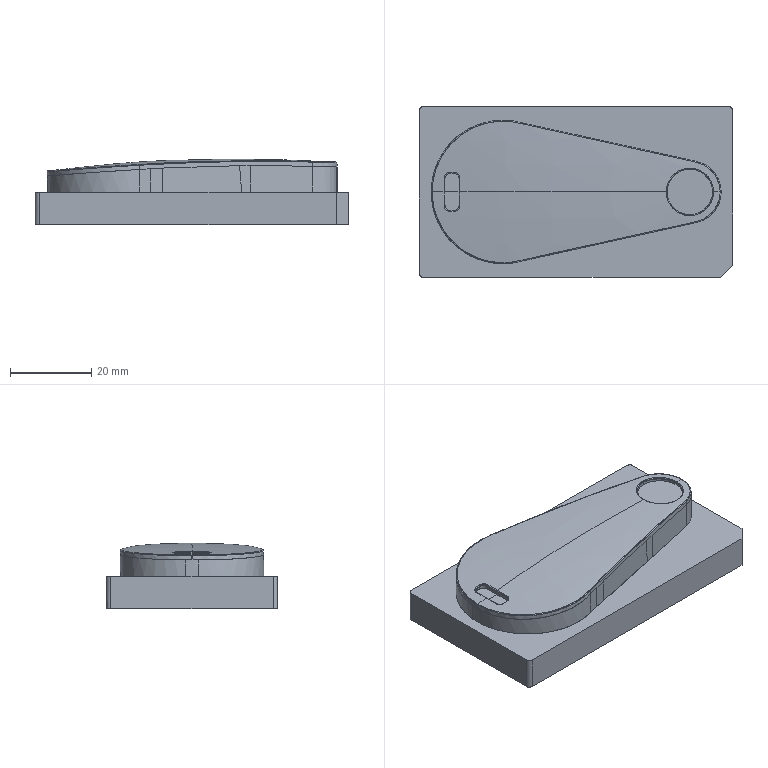NC program | PowerMill | posted with a generic post | part box 77 x 42 x 16.114 mm
Lines 17525 to 19132 of 230441, first 1450 of 1608 lines:
N17622 M6
N17623 S18000 M03
N17624 G00 G90 X0.0 Y0.0
N17625 G43 Z9.8037 H28
N17626
N17627 G05 P10000 R4
N17628 X-29.8878 Y2.5312
N17629 Z-1.421
N17630 G01 Z-2.621 F2400.0
N17631 X-29.8713 Y2.5316 F4000.0
N17632 G03 X-29.726 Y2.6832 I-0.0032 J0.1484
N17633 G01 X-29.7401 Y3.336
N17634 X-29.7435 Y3.3599
N17635 X-29.7525 Y3.3822
N17636 X-29.8269 Y3.5167
N17637 X-29.8421 Y3.5374
N17638 X-29.8621 Y3.5535
N17639 X-29.9916 Y3.633
N17640 X-30.0319 Y3.647
N17641 X-30.5975 Y3.7149
N17642 X-29.8892 Y2.3639 Z-2.7177
N17643 X-29.8727
N17644 G03 X-29.7242 Y2.5124 I0.0 J0.1485
N17645 G01 Y2.5785
N17646 X-29.7405 Y3.335
N17647 X-29.7439 Y3.359
N17648 X-29.753 Y3.3814
N17649 X-29.8258 Y3.5126
N17650 X-29.8424 Y3.5347
N17651 X-29.8644 Y3.5514
N17652 X-29.9942 Y3.6241
N17653 X-30.0167 Y3.6334
N17654 X-30.0408 Y3.6369
N17655 X-30.827 Y3.6548
N17656 G00 Z1.579
N17657 G01 X-30.7616 Y-3.5711 F10000.0
N17658 G00 Z-1.421
N17659 G01 Z-2.621 F2400.0
N17660 X-30.7596 Y-3.5875 F4000.0
N17661 G03 X-30.5941 Y-3.7167 I0.1474 J0.0182
N17662 G01 X-30.0322 Y-3.6476
N17663 X-29.9918 Y-3.6335
N17664 X-29.8615 Y-3.553
N17665 X-29.8417 Y-3.5368
N17666 X-29.8266 Y-3.5162
N17667 X-29.7519 Y-3.3811
N17668 X-29.7431 Y-3.3596
N17669 X-29.7263 Y-3.0196
N17670 X-29.7252 Y-2.6792
N17671 X-30.9888 Y-3.4914 Z-2.7177
N17672 X-30.9886 Y-3.5079
N17673 G03 X-30.8387 Y-3.655 I0.1485 J0.0014
N17674 G01 X-30.0951 Y-3.6479
N17675 X-29.9745 Y-3.6175
N17676 X-29.9604 Y-3.6128
N17677 X-29.9472 Y-3.606
N17678 X-29.9065 Y-3.5808
N17679 X-29.8454 Y-3.5337
N17680 X-29.831 Y-3.5201
N17681 X-29.8196 Y-3.5038
N17682 X-29.7549 Y-3.3866
N17683 X-29.7484 Y-3.3722
N17684 X-29.7444 Y-3.3569
N17685 X-29.7248 Y-2.9283
N17686 X-29.7249 Y-2.4993
N17687 X-31.2076 Y-2.5192 Z-2.6145
N17688 X-31.2074 Y-3.3335 Z-2.6287 F2400.0
N17689 X-31.1952 Y-3.373 Z-2.6294
N17690 X-31.097 Y-3.5168 Z-2.6325
N17691 X-31.0697 Y-3.5403 Z-2.6331
N17692 X-30.9489 Y-3.599 Z-2.6354
N17693 X-30.9192 Y-3.606 Z-2.636
N17694 X-30.0987 Y-3.6169 Z-2.6503
N17695 X-29.9719 Y-3.5858 Z-2.6526
N17696 X-29.9713 Y-3.5856
N17697 X-29.924 Y-3.5564 Z-2.6535
N17698 X-29.8574 Y-3.5051 Z-2.655
N17699 X-29.8521 Y-3.5006 Z-2.6551
N17700 X-29.7781 Y-3.3667 Z-2.6578
N17701 X-29.7752 Y-3.3606 Z-2.6579
N17702 X-29.772 Y-3.3426 Z-2.6582
N17703 X-29.7555 Y-2.9522 Z-2.6651
N17704 X-29.7549 Y-2.4993 Z-2.673
N17705 X-29.7542 Y-2.0587 Z-2.6806
N17706 Y-0.6131 Z-2.7059
N17707 X-29.9539 Z-2.7094
N17708 X-30.3986 Y-0.7228 Z-2.7174
N17709 X-30.8042 Y-0.9356 Z-2.7253
N17710 X-31.147 Y-1.2394 Z-2.7333
N17711 X-31.2079 Y-1.3275 Z-2.7352
N17712 X-31.2074 Y-3.3335 Z-2.7702
N17713 X-31.1952 Y-3.373 Z-2.7709
N17714 X-31.097 Y-3.5168 Z-2.774
N17715 X-31.0697 Y-3.5403 Z-2.7746
N17716 X-30.9489 Y-3.599 Z-2.7769
N17717 X-30.9192 Y-3.606 Z-2.7775
N17718 X-30.0987 Y-3.6169 Z-2.7918
N17719 X-29.9719 Y-3.5858 Z-2.7941
N17720 X-29.9713 Y-3.5856
N17721 X-29.924 Y-3.5564 Z-2.7951
N17722 X-29.8574 Y-3.5051 Z-2.7965
N17723 X-29.8521 Y-3.5006 Z-2.7966
N17724 X-29.7781 Y-3.3667 Z-2.7993
N17725 X-29.7752 Y-3.3606 Z-2.7994
N17726 X-29.772 Y-3.3426 Z-2.7998
N17727 X-29.7555 Y-2.9522 Z-2.8066
N17728 X-29.7549 Y-2.4993 Z-2.8145
N17729 X-29.7249
N17730 X-29.7242 Y-2.0587 F4000.0
N17731 Y2.5785
N17732 X-29.7243 Y2.5825
N17733 X-29.7398 Y3.3077
N17734 X-29.7659 Y3.4048
N17735 X-29.8139 Y3.4913
N17736 X-29.8799 Y3.5601
N17737 X-29.9667 Y3.6088
N17738 X-30.0627 Y3.6374
N17739 X-30.3495 Y3.644
N17740 X-30.919 Y3.6369
N17741 X-30.9413 Y3.6341
N17742 X-30.9624 Y3.6264
N17743 X-31.0855 Y3.5651
N17744 X-31.1064 Y3.5511
N17745 X-31.1232 Y3.5324
N17746 X-31.2212 Y3.3903
N17747 X-31.2344 Y3.3632
N17748 X-31.2389 Y3.3335
N17749 X-31.2374 Y-3.3335
N17750 X-31.2329 Y-3.363
N17751 X-31.22 Y-3.3899
N17752 X-31.1218 Y-3.5337
N17753 X-31.1045 Y-3.5531
N17754 X-31.0828 Y-3.5673
N17755 X-30.9619 Y-3.626
N17756 X-30.9413 Y-3.6333
N17757 X-30.9197 Y-3.636
N17758 X-30.0953 Y-3.647
N17759 X-29.9648 Y-3.6149
N17760 X-29.9619 Y-3.6142
N17761 X-29.959 Y-3.6133
N17762 X-29.907 Y-3.5811
N17763 X-29.8391 Y-3.5289
N17764 X-29.8334 Y-3.5242
N17765 X-29.8281 Y-3.519
N17766 X-29.8272 Y-3.5177
N17767 X-29.8265 Y-3.5163
N17768 X-29.7519 Y-3.3812
N17769 X-29.7493 Y-3.3762
N17770 X-29.747 Y-3.3711
N17771 X-29.7436 Y-3.3577
N17772 X-29.742 Y-3.3438
N17773 X-29.7255 Y-2.9528
N17774 X-29.7249 Y-2.4993
N17775 X-31.1785 Y-2.4363 Z-2.7112
N17776 X-31.1788 Y-3.2629 Z-2.7257 F2400.0
N17777 X-31.1515 Y-3.3898 Z-2.7279
N17778 X-31.1378 Y-3.4188 Z-2.7285
N17779 X-31.0478 Y-3.5314 Z-2.731
N17780 X-30.9867 Y-3.5716 Z-2.7323
N17781 X-30.956 Y-3.5828 Z-2.7329
N17782 X-30.7255 Y-3.6086 Z-2.7369
N17783 X-30.0989 Y-3.617 Z-2.7478
N17784 X-29.9719 Y-3.5858 Z-2.7501
N17785 X-29.9711 Y-3.5856
N17786 X-29.9245 Y-3.5568 Z-2.7511
N17787 X-29.8574 Y-3.5051 Z-2.7526
N17788 X-29.852 Y-3.5005 Z-2.7527
N17789 X-29.7781 Y-3.3667 Z-2.7554
N17790 X-29.7753 Y-3.3611 Z-2.7555
N17791 X-29.772 Y-3.3426 Z-2.7558
N17792 X-29.7555 Y-2.9507 Z-2.7626
N17793 X-29.7548 Y-2.4993 Z-2.7705
N17794 X-29.7542 Y-2.1026 Z-2.7774
N17795 Y-0.6131 Z-2.8034
N17796 X-29.9538 Z-2.8069
N17797 X-30.3986 Y-0.7228 Z-2.8149
N17798 X-30.8041 Y-0.9356 Z-2.8229
N17799 X-31.147 Y-1.2394 Z-2.8309
N17800 X-31.1782 Y-1.2845 Z-2.8319
N17801 X-31.1788 Y-3.2629 Z-2.8664
N17802 X-31.1515 Y-3.3898 Z-2.8687
N17803 X-31.1378 Y-3.4188 Z-2.8692
N17804 X-31.0478 Y-3.5314 Z-2.8717
N17805 X-30.9867 Y-3.5716 Z-2.873
N17806 X-30.956 Y-3.5828 Z-2.8736
N17807 X-30.7255 Y-3.6086 Z-2.8776
N17808 X-30.0989 Y-3.617 Z-2.8886
N17809 X-29.9719 Y-3.5858 Z-2.8908
N17810 X-29.9711 Y-3.5856 Z-2.8909
N17811 X-29.9245 Y-3.5568 Z-2.8918
N17812 X-29.8574 Y-3.5051 Z-2.8933
N17813 X-29.852 Y-3.5005 Z-2.8934
N17814 X-29.7781 Y-3.3667 Z-2.8961
N17815 X-29.7753 Y-3.3611 Z-2.8962
N17816 X-29.772 Y-3.3426 Z-2.8965
N17817 X-29.7555 Y-2.9507 Z-2.9034
N17818 X-29.7548 Y-2.4993 Z-2.9112
N17819 X-29.7248
N17820 X-29.7242 Y-2.1027 F4000.0
N17821 X-29.7243 Y2.5785
N17822 X-29.7399 Y3.3081
N17823 X-29.7658 Y3.4044
N17824 X-29.8141 Y3.4916
N17825 X-29.8794 Y3.5597
N17826 X-29.9684 Y3.6093
N17827 X-30.0617 Y3.6372
N17828 X-30.103 Y3.6384
N17829 X-30.3495 Y3.644
N17830 X-30.7191 Y3.6394
N17831 X-30.9522 Y3.6133
N17832 X-30.9811 Y3.6056
N17833 X-31.0065 Y3.5896
N17834 X-31.1417 Y3.4724
N17835 X-31.185 Y3.3872
N17836 X-31.193 Y3.3655
N17837 X-31.1959 Y3.3427
N17838 X-31.2071 Y1.8909
N17839 X-31.2088 Y-3.2661
N17840 X-31.1809 Y-3.3961
N17841 X-31.1734 Y-3.418
N17842 X-31.1612 Y-3.4376
N17843 X-31.0682 Y-3.5538
N17844 X-31.0032 Y-3.5967
N17845 X-30.9822 Y-3.6072
N17846 X-30.9593 Y-3.6126
N17847 X-30.7274 Y-3.6386
N17848 X-30.0973 Y-3.647
N17849 X-30.0952
N17850 X-29.9648 Y-3.6149
N17851 X-29.9618 Y-3.6141
N17852 X-29.9588 Y-3.6133
N17853 X-29.9074 Y-3.5815
N17854 X-29.8391 Y-3.5289
N17855 X-29.8333 Y-3.5241
N17856 X-29.8279 Y-3.5189
N17857 X-29.8272 Y-3.5176
N17858 X-29.8264 Y-3.5163
N17859 X-29.7518 Y-3.3812
N17860 X-29.7494 Y-3.3765
N17861 X-29.7472 Y-3.3718
N17862 X-29.7436 Y-3.358
N17863 X-29.742 Y-3.3438
N17864 X-29.7255 Y-2.9513
N17865 X-29.7248 Y-2.4993
N17866 X-31.1716 Y-2.4142 Z-2.808
N17867 Y-2.5782 Z-2.8109 F2400.0
N17868 X-31.1549 Y-3.359 Z-2.8245
N17869 X-31.1199 Y-3.4375 Z-2.826
N17870 X-31.1026 Y-3.4612 Z-2.8265
N17871 X-30.985 Y-3.5663 Z-2.8292
N17872 X-30.9462 Y-3.5836 Z-2.83
N17873 X-30.7242 Y-3.6087 Z-2.8339
N17874 X-30.0992 Y-3.617 Z-2.8448
N17875 X-30.0991
N17876 X-29.9719 Y-3.5858 Z-2.8471
N17877 X-29.9709 Y-3.5855
N17878 X-29.9249 Y-3.5571 Z-2.848
N17879 X-29.8574 Y-3.5051 Z-2.8495
N17880 X-29.8519 Y-3.5004 Z-2.8497
N17881 X-29.778 Y-3.3667 Z-2.8523
N17882 X-29.7755 Y-3.3616 Z-2.8524
N17883 X-29.772 Y-3.3426 Z-2.8528
N17884 X-29.7554 Y-2.9492 Z-2.8596
N17885 X-29.7548 Y-2.4993 Z-2.8675
N17886 X-29.7543 Y-2.1452 Z-2.8737
N17887 Y-0.6131 Z-2.9004
N17888 X-29.9538 Z-2.9039
N17889 X-30.3985 Y-0.7228 Z-2.9119
N17890 X-30.8041 Y-0.9356 Z-2.9199
N17891 X-31.1469 Y-1.2394 Z-2.9279
N17892 X-31.1712 Y-1.2746 Z-2.9286
N17893 X-31.1716 Y-2.5782 Z-2.9514
N17894 X-31.1549 Y-3.359 Z-2.965
N17895 X-31.1199 Y-3.4375 Z-2.9665
N17896 X-31.1026 Y-3.4612 Z-2.967
N17897 X-30.985 Y-3.5663 Z-2.9698
N17898 X-30.9462 Y-3.5836 Z-2.9705
N17899 X-30.7242 Y-3.6087 Z-2.9744
N17900 X-30.0992 Y-3.617 Z-2.9853
N17901 X-30.0991
N17902 X-29.9719 Y-3.5858 Z-2.9876
N17903 X-29.9709 Y-3.5855
N17904 X-29.9249 Y-3.5571 Z-2.9886
N17905 X-29.8574 Y-3.5051 Z-2.99
N17906 X-29.8519 Y-3.5004 Z-2.9902
N17907 X-29.778 Y-3.3667 Z-2.9928
N17908 X-29.7755 Y-3.3616 Z-2.9929
N17909 X-29.772 Y-3.3426 Z-2.9933
N17910 X-29.7554 Y-2.9492 Z-3.0001
N17911 X-29.7548 Y-2.4993 Z-3.008
N17912 X-29.7248
N17913 X-29.7243 Y-2.1453 F4000.0
N17914 Y2.5785
N17915 X-29.7399 Y3.3083
N17916 X-29.7657 Y3.4042
N17917 X-29.8142 Y3.4918
N17918 X-29.8793 Y3.5596
N17919 X-29.9686 Y3.6095
N17920 X-30.0616 Y3.6372
N17921 X-30.1102 Y3.6386
N17922 X-30.3495 Y3.6441
N17923 X-30.7179 Y3.6395
N17924 X-30.9496 Y3.6135
N17925 X-30.9793 Y3.6054
N17926 X-31.0051 Y3.5886
N17927 X-31.1177 Y3.4878
N17928 X-31.1354 Y3.467
N17929 X-31.1468 Y3.4422
N17930 X-31.1964 Y3.2778
N17931 X-31.2001 Y2.8058
N17932 X-31.2016 Y-2.5785
N17933 X-31.1847 Y-3.3656
N17934 X-31.1473 Y-3.4497
N17935 X-31.1367 Y-3.4679
N17936 X-31.1226 Y-3.4836
N17937 X-31.0049 Y-3.5887
N17938 X-30.9792 Y-3.6054
N17939 X-30.9495 Y-3.6135
N17940 X-30.726 Y-3.6387
N17941 X-30.0992 Y-3.647
N17942 X-30.0953
N17943 X-29.9648 Y-3.6149
N17944 X-29.9617 Y-3.6141
N17945 X-29.9586 Y-3.6132
N17946 X-29.9078 Y-3.5818
N17947 X-29.8391 Y-3.5289
N17948 X-29.8332 Y-3.524
N17949 X-29.8278 Y-3.5187
N17950 X-29.8271 Y-3.5175
N17951 X-29.8264 Y-3.5163
N17952 X-29.7518 Y-3.3812
N17953 X-29.7495 Y-3.3769
N17954 X-29.7475 Y-3.3724
N17955 X-29.7437 Y-3.3583
N17956 X-29.742 Y-3.3438
N17957 X-29.7254 Y-2.9498
N17958 X-29.7248 Y-2.4993
N17959 X-31.1714 Y-2.4074 Z-2.9047
N17960 Y-2.5784 Z-2.9077 F2400.0
N17961 X-31.1713 Y-2.5954 Z-2.908
N17962 X-31.1562 Y-3.2986 Z-2.9203
N17963 X-31.1168 Y-3.4349 Z-2.9228
N17964 X-31.1022 Y-3.4616 Z-2.9233
N17965 X-30.985 Y-3.5663 Z-2.9261
N17966 X-30.969 Y-3.5771 Z-2.9264
N17967 X-30.9463 Y-3.5836 Z-2.9268
N17968 X-30.7235 Y-3.6087 Z-2.9307
N17969 X-30.1012 Y-3.6171 Z-2.9416
N17970 X-30.0991 Y-3.617
N17971 X-29.9719 Y-3.5858 Z-2.9439
N17972 X-29.9708 Y-3.5855
N17973 X-29.9253 Y-3.5574 Z-2.9449
N17974 X-29.8574 Y-3.5051 Z-2.9464
N17975 X-29.8517 Y-3.5003 Z-2.9465
N17976 X-29.778 Y-3.3667 Z-2.9491
N17977 X-29.7756 Y-3.362 Z-2.9492
N17978 X-29.772 Y-3.3426 Z-2.9496
N17979 X-29.7554 Y-2.9476 Z-2.9565
N17980 X-29.7547 Y-2.4993 Z-2.9643
N17981 X-29.7543 Y-2.1892 Z-2.9697
N17982 Y-0.6131 Z-2.9972
N17983 X-29.9537 Z-3.0007
N17984 X-30.3985 Y-0.7228 Z-3.0087
N17985 X-30.804 Y-0.9356 Z-3.0167
N17986 X-31.1469 Y-1.2394 Z-3.0247
N17987 X-31.171 Y-1.2743 Z-3.0254
N17988 X-31.1714 Y-2.5784 Z-3.0482
N17989 X-31.1713 Y-2.5954 Z-3.0485
N17990 X-31.1562 Y-3.2986 Z-3.0608
N17991 X-31.1168 Y-3.4349 Z-3.0632
N17992 X-31.1022 Y-3.4616 Z-3.0638
N17993 X-30.985 Y-3.5663 Z-3.0665
N17994 X-30.969 Y-3.5771 Z-3.0668
N17995 X-30.9463 Y-3.5836 Z-3.0673
N17996 X-30.7235 Y-3.6087 Z-3.0712
N17997 X-30.1012 Y-3.6171 Z-3.082
N17998 X-30.0991 Y-3.617 Z-3.0821
N17999 X-29.9719 Y-3.5858 Z-3.0843
N18000 X-29.9708 Y-3.5855 Z-3.0844
N18001 X-29.9253 Y-3.5574 Z-3.0853
N18002 X-29.8574 Y-3.5051 Z-3.0868
N18003 X-29.8517 Y-3.5003 Z-3.0869
N18004 X-29.778 Y-3.3667 Z-3.0896
N18005 X-29.7756 Y-3.362 Z-3.0897
N18006 X-29.772 Y-3.3426 Z-3.09
N18007 X-29.7554 Y-2.9476 Z-3.0969
N18008 X-29.7547 Y-2.4993 Z-3.1047
N18009 X-29.7247
N18010 X-29.7243 Y-2.1892 F4000.0
N18011 Y2.5785
N18012 X-29.7399 Y3.3085
N18013 X-29.7656 Y3.404
N18014 X-29.8143 Y3.4919
N18015 X-29.8791 Y3.5595
N18016 X-29.9689 Y3.6096
N18017 X-30.0614 Y3.6372
N18018 X-30.1175 Y3.6388
N18019 X-30.3495 Y3.6441
N18020 X-30.7172 Y3.6396
N18021 X-30.9495 Y3.6135
N18022 X-30.9792 Y3.6054
N18023 X-31.0051 Y3.5886
N18024 X-31.1177 Y3.4878
N18025 X-31.1354 Y3.4669
N18026 X-31.1468 Y3.442
N18027 X-31.1965 Y3.2761
N18028 X-31.1996 Y2.8745
N18029 X-31.2014 Y-2.5785
N18030 X-31.2013 Y-2.5958
N18031 X-31.1861 Y-3.3032
N18032 X-31.1457 Y-3.4432
N18033 X-31.1369 Y-3.4643
N18034 X-31.1235 Y-3.4828
N18035 X-31.1231 Y-3.4832
N18036 X-31.1226 Y-3.4836
N18037 X-31.005 Y-3.5887
N18038 X-30.9941 Y-3.5972
N18039 X-30.9821 Y-3.604
N18040 X-30.9663 Y-3.6101
N18041 X-30.9497 Y-3.6134
N18042 X-30.7254 Y-3.6387
N18043 X-30.1012 Y-3.6471
N18044 X-30.0953 Y-3.647
N18045 X-29.9648 Y-3.6149
N18046 X-29.9616 Y-3.6141
N18047 X-29.9584 Y-3.6131
N18048 X-29.9083 Y-3.5821
N18049 X-29.8391 Y-3.5289
N18050 X-29.8332 Y-3.524
N18051 X-29.8276 Y-3.5186
N18052 X-29.8263 Y-3.5163
N18053 X-29.7517 Y-3.3812
N18054 X-29.7496 Y-3.3772
N18055 X-29.7477 Y-3.3731
N18056 X-29.7438 Y-3.3587
N18057 X-29.742 Y-3.3439
N18058 X-29.7254 Y-2.9483
N18059 X-29.7247 Y-2.4993
N18060 X-31.1713 Y-2.4064 Z-3.0015
N18061 X-31.1714 Y-2.5784 Z-3.0045 F2400.0
N18062 X-31.1712 Y-2.6002 Z-3.0049
N18063 X-31.1563 Y-3.2984 Z-3.0171
N18064 X-31.1168 Y-3.4349 Z-3.0195
N18065 X-31.102 Y-3.4618 Z-3.0201
N18066 X-30.9898 Y-3.5621 Z-3.0227
N18067 X-30.9849 Y-3.5664 Z-3.0228
N18068 X-30.9463 Y-3.5836 Z-3.0236
N18069 X-30.7229 Y-3.6088 Z-3.0275
N18070 X-30.1031 Y-3.6171 Z-3.0383
N18071 X-30.0991 Y-3.617 Z-3.0384
N18072 X-29.972 Y-3.5858 Z-3.0407
N18073 X-29.9706 Y-3.5854
N18074 X-29.9258 Y-3.5577 Z-3.0416
N18075 X-29.8574 Y-3.5052 Z-3.0431
N18076 X-29.8516 Y-3.5002 Z-3.0432
N18077 X-29.7779 Y-3.3667 Z-3.0459
N18078 X-29.7758 Y-3.3625 Z-3.046
N18079 X-29.772 Y-3.3426 Z-3.0463
N18080 X-29.7553 Y-2.9461 Z-3.0533
N18081 X-29.7547 Y-2.4993 Z-3.0611
N18082 X-29.7543 Y-2.2318 Z-3.0657
N18083 Y-0.6131 Z-3.094
N18084 X-29.9537 Z-3.0975
N18085 X-30.3984 Y-0.7228 Z-3.1055
N18086 X-30.804 Y-0.9356 Z-3.1134
N18087 X-31.1468 Y-1.2394 Z-3.1214
N18088 X-31.171 Y-1.2743 Z-3.1222
N18089 X-31.1714 Y-2.5784 Z-3.1449
N18090 X-31.1712 Y-2.6002 Z-3.1453
N18091 X-31.1563 Y-3.2984 Z-3.1575
N18092 X-31.1168 Y-3.4349 Z-3.16
N18093 X-31.102 Y-3.4618 Z-3.1605
N18094 X-30.9898 Y-3.5621 Z-3.1631
N18095 X-30.9849 Y-3.5664 Z-3.1633
N18096 X-30.9463 Y-3.5836 Z-3.164
N18097 X-30.7229 Y-3.6088 Z-3.1679
N18098 X-30.1031 Y-3.6171 Z-3.1787
N18099 X-30.0991 Y-3.617 Z-3.1788
N18100 X-29.972 Y-3.5858 Z-3.1811
N18101 X-29.9706 Y-3.5854
N18102 X-29.9258 Y-3.5577 Z-3.182
N18103 X-29.8574 Y-3.5052 Z-3.1835
N18104 X-29.8516 Y-3.5002 Z-3.1837
N18105 X-29.7779 Y-3.3667 Z-3.1863
N18106 X-29.7758 Y-3.3625 Z-3.1864
N18107 X-29.772 Y-3.3426 Z-3.1868
N18108 X-29.7553 Y-2.9461 Z-3.1937
N18109 X-29.7547 Y-2.4993 Z-3.2015
N18110 X-29.7247
N18111 X-29.7243 Y-2.2318 F4000.0
N18112 Y2.5785
N18113 X-29.7399 Y3.3087
N18114 X-29.7655 Y3.4038
N18115 X-29.8144 Y3.4921
N18116 X-29.8789 Y3.5594
N18117 X-29.9691 Y3.6097
N18118 X-30.0612 Y3.6372
N18119 X-30.1249 Y3.639
N18120 X-30.3495 Y3.6442
N18121 X-30.7166 Y3.6396
N18122 X-30.9495 Y3.6135
N18123 X-30.9792 Y3.6054
N18124 X-31.005 Y3.5886
N18125 X-31.1177 Y3.4879
N18126 X-31.1354 Y3.4669
N18127 X-31.1468 Y3.442
N18128 X-31.1965 Y3.2758
N18129 X-31.1996 Y2.8843
N18130 X-31.2014 Y-2.5785
N18131 X-31.2012 Y-2.6006
N18132 X-31.1862 Y-3.3029
N18133 X-31.1457 Y-3.4432
N18134 X-31.1368 Y-3.4645
N18135 X-31.1232 Y-3.4831
N18136 X-31.0097 Y-3.5845
N18137 X-31.0048 Y-3.5889
N18138 X-30.9791 Y-3.6054
N18139 X-30.9497 Y-3.6134
N18140 X-30.7248 Y-3.6388
N18141 X-30.1031 Y-3.6471
N18142 X-30.0953 Y-3.647
N18143 X-29.9648 Y-3.6149
N18144 X-29.9615 Y-3.614
N18145 X-29.9582 Y-3.6131
N18146 X-29.9087 Y-3.5824
N18147 X-29.8391 Y-3.5289
N18148 X-29.8331 Y-3.5239
N18149 X-29.8275 Y-3.5184
N18150 X-29.8263 Y-3.5164
N18151 X-29.7517 Y-3.3813
N18152 X-29.7497 Y-3.3775
N18153 X-29.7479 Y-3.3737
N18154 X-29.7438 Y-3.359
N18155 X-29.742 Y-3.3439
N18156 X-29.7253 Y-2.9468
N18157 X-29.7247 Y-2.4993
N18158 X-31.1713 Y-2.4063 Z-3.0983
N18159 X-31.1714 Y-2.5784 Z-3.1013 F2400.0
N18160 X-31.1712 Y-2.605 Z-3.1017
N18161 X-31.1563 Y-3.2981 Z-3.1138
N18162 X-31.1168 Y-3.4349 Z-3.1163
N18163 X-31.1017 Y-3.4622 Z-3.1169
N18164 X-31.0026 Y-3.5507 Z-3.1192
N18165 X-30.9849 Y-3.5664 Z-3.1196
N18166 X-30.9463 Y-3.5836 Z-3.1203
N18167 X-30.7223 Y-3.6088 Z-3.1243
N18168 X-30.1051 Y-3.6171 Z-3.135
N18169 X-30.0991 Y-3.617 Z-3.1351
N18170 X-29.972 Y-3.5858 Z-3.1374
N18171 X-29.9704 Y-3.5854
N18172 X-29.9262 Y-3.5581 Z-3.1384
N18173 X-29.8574 Y-3.5052 Z-3.1399
N18174 X-29.8515 Y-3.5001 Z-3.14
N18175 X-29.7779 Y-3.3668 Z-3.1427
N18176 X-29.7759 Y-3.3629
N18177 X-29.772 Y-3.3426 Z-3.1431
N18178 X-29.7553 Y-2.9446 Z-3.1501
N18179 X-29.7546 Y-2.4993 Z-3.1578
N18180 X-29.7543 Y-2.2757 Z-3.1617
N18181 Y-0.6131 Z-3.1907
N18182 X-29.9536 Z-3.1942
N18183 X-30.3984 Y-0.7228 Z-3.2022
N18184 X-30.8039 Y-0.9356 Z-3.2102
N18185 X-31.1468 Y-1.2394 Z-3.2182
N18186 X-31.1709 Y-1.2743 Z-3.2189
N18187 X-31.1714 Y-2.5784 Z-3.2417
N18188 X-31.1712 Y-2.605 Z-3.2422
N18189 X-31.1563 Y-3.2981 Z-3.2543
N18190 X-31.1168 Y-3.4349 Z-3.2567
N18191 X-31.1017 Y-3.4622 Z-3.2573
N18192 X-31.0026 Y-3.5507 Z-3.2596
N18193 X-30.9849 Y-3.5664 Z-3.26
N18194 X-30.9463 Y-3.5836 Z-3.2608
N18195 X-30.7223 Y-3.6088 Z-3.2647
N18196 X-30.1051 Y-3.6171 Z-3.2755
N18197 X-30.0991 Y-3.617 Z-3.2756
N18198 X-29.972 Y-3.5858 Z-3.2779
N18199 X-29.9704 Y-3.5854
N18200 X-29.9262 Y-3.5581 Z-3.2788
N18201 X-29.8574 Y-3.5052 Z-3.2803
N18202 X-29.8515 Y-3.5001 Z-3.2804
N18203 X-29.7779 Y-3.3668 Z-3.2831
N18204 X-29.7759 Y-3.3629 Z-3.2832
N18205 X-29.772 Y-3.3426 Z-3.2835
N18206 X-29.7553 Y-2.9446 Z-3.2905
N18207 X-29.7546 Y-2.4993 Z-3.2983
N18208 X-29.7246
N18209 X-29.7243 Y-2.2757 F4000.0
N18210 Y2.5785
N18211 X-29.7399 Y3.3089
N18212 X-29.7654 Y3.4037
N18213 X-29.8145 Y3.4923
N18214 X-29.8787 Y3.5592
N18215 X-29.9693 Y3.6098
N18216 X-30.061 Y3.6372
N18217 X-30.1325 Y3.6393
N18218 X-30.3495 Y3.6442
N18219 X-30.716 Y3.6397
N18220 X-30.9495 Y3.6135
N18221 X-30.9792 Y3.6054
N18222 X-31.005 Y3.5886
N18223 X-31.1176 Y3.4879
N18224 X-31.1354 Y3.467
N18225 X-31.1468 Y3.442
N18226 X-31.1966 Y3.2756
N18227 X-31.1995 Y2.894
N18228 X-31.2014 Y-2.5785
N18229 X-31.2012 Y-2.6054
N18230 X-31.1862 Y-3.3027
N18231 X-31.1457 Y-3.4432
N18232 X-31.1366 Y-3.4647
N18233 X-31.1229 Y-3.4835
N18234 X-31.0226 Y-3.5731
N18235 X-31.0048 Y-3.5889
N18236 X-30.9791 Y-3.6054
N18237 X-30.9496 Y-3.6134
N18238 X-30.7242 Y-3.6388
N18239 X-30.1051 Y-3.6471
N18240 X-30.0953 Y-3.647
N18241 X-29.9648 Y-3.6149
N18242 X-29.9614 Y-3.614
N18243 X-29.958 Y-3.613
N18244 X-29.9091 Y-3.5828
N18245 X-29.8391 Y-3.5289
N18246 X-29.833 Y-3.5238
N18247 X-29.8273 Y-3.5183
N18248 X-29.8262 Y-3.5164
N18249 X-29.7516 Y-3.3813
N18250 X-29.7498 Y-3.3779
N18251 X-29.7482 Y-3.3744
N18252 X-29.7439 Y-3.3594
N18253 X-29.742 Y-3.3439
N18254 X-29.7253 Y-2.9452
N18255 X-29.7246 Y-2.4993
N18256 X-31.1713 Y-2.4063 Z-3.195
N18257 Y-2.5784 Z-3.198 F2400.0
N18258 X-31.1711 Y-2.6098 Z-3.1986
N18259 X-31.1564 Y-3.2978 Z-3.2106
N18260 X-31.1168 Y-3.4349 Z-3.2131
N18261 X-31.1014 Y-3.4625 Z-3.2136
N18262 X-31.015 Y-3.5397 Z-3.2156
N18263 X-30.9849 Y-3.5664 Z-3.2163
N18264 X-30.9463 Y-3.5836 Z-3.2171
N18265 X-30.7217 Y-3.6089 Z-3.221
N18266 X-30.107 Y-3.6171 Z-3.2317
N18267 X-30.0991 Y-3.617 Z-3.2319
N18268 X-29.972 Y-3.5858 Z-3.2342
N18269 X-29.9702 Y-3.5853
N18270 X-29.9266 Y-3.5584 Z-3.2351
N18271 X-29.8574 Y-3.5052 Z-3.2366
N18272 X-29.8514 Y-3.5 Z-3.2368
N18273 X-29.7779 Y-3.3668 Z-3.2394
N18274 X-29.7761 Y-3.3634 Z-3.2395
N18275 X-29.772 Y-3.3426 Z-3.2399
N18276 X-29.7552 Y-2.9431 Z-3.2468
N18277 X-29.7546 Y-2.4993 Z-3.2546
N18278 X-29.7543 Y-2.3183 Z-3.2577
N18279 Y-0.6131 Z-3.2875
N18280 X-29.9536 Z-3.291
N18281 X-30.3983 Y-0.7228 Z-3.299
N18282 X-30.8039 Y-0.9356 Z-3.307
N18283 X-31.1467 Y-1.2394 Z-3.3149
N18284 X-31.1709 Y-1.2744 Z-3.3157
N18285 X-31.1713 Y-2.5784 Z-3.3384
N18286 X-31.1711 Y-2.6098 Z-3.339
N18287 X-31.1564 Y-3.2978 Z-3.351
N18288 X-31.1168 Y-3.4349 Z-3.3535
N18289 X-31.1014 Y-3.4625 Z-3.354
N18290 X-31.015 Y-3.5397 Z-3.3561
N18291 X-30.9849 Y-3.5664 Z-3.3568
N18292 X-30.9463 Y-3.5836 Z-3.3575
N18293 X-30.7217 Y-3.6089 Z-3.3615
N18294 X-30.107 Y-3.6171 Z-3.3722
N18295 X-30.0991 Y-3.617 Z-3.3723
N18296 X-29.972 Y-3.5858 Z-3.3746
N18297 X-29.9702 Y-3.5853
N18298 X-29.9266 Y-3.5584 Z-3.3755
N18299 X-29.8574 Y-3.5052 Z-3.3771
N18300 X-29.8514 Y-3.5 Z-3.3772
N18301 X-29.7779 Y-3.3668 Z-3.3798
N18302 X-29.7761 Y-3.3634 Z-3.3799
N18303 X-29.772 Y-3.3426 Z-3.3803
N18304 X-29.7552 Y-2.9431 Z-3.3873
N18305 X-29.7546 Y-2.4993 Z-3.395
N18306 X-29.7246
N18307 X-29.7243 Y-2.3183 F4000.0
N18308 Y2.5785
N18309 X-29.7399 Y3.3091
N18310 X-29.7653 Y3.4035
N18311 X-29.8146 Y3.4924
N18312 X-29.8786 Y3.5591
N18313 X-29.9695 Y3.6099
N18314 X-30.0608 Y3.6372
N18315 X-30.14 Y3.6395
N18316 X-30.3495 Y3.6443
N18317 X-30.7154 Y3.6397
N18318 X-30.9495 Y3.6135
N18319 X-30.9792 Y3.6054
N18320 X-31.005 Y3.5886
N18321 X-31.1176 Y3.4879
N18322 X-31.1354 Y3.467
N18323 X-31.1468 Y3.442
N18324 X-31.1966 Y3.2753
N18325 X-31.1995 Y2.9038
N18326 X-31.2013 Y-2.5785
N18327 X-31.2011 Y-2.6102
N18328 X-31.1863 Y-3.3024
N18329 X-31.1457 Y-3.4432
N18330 X-31.1365 Y-3.4649
N18331 X-31.1225 Y-3.4839
N18332 X-31.035 Y-3.5621
N18333 X-31.0048 Y-3.5889
N18334 X-30.9791 Y-3.6054
N18335 X-30.9496 Y-3.6134
N18336 X-30.7236 Y-3.6389
N18337 X-30.1071 Y-3.6471
N18338 X-30.0953 Y-3.647
N18339 X-29.9648 Y-3.6149
N18340 X-29.9613 Y-3.614
N18341 X-29.9578 Y-3.6129
N18342 X-29.9096 Y-3.5831
N18343 X-29.8391 Y-3.5289
N18344 X-29.8329 Y-3.5238
N18345 X-29.8272 Y-3.5181
N18346 X-29.8262 Y-3.5164
N18347 X-29.7516 Y-3.3813
N18348 X-29.7499 Y-3.3782
N18349 X-29.7484 Y-3.375
N18350 X-29.744 Y-3.3597
N18351 X-29.742 Y-3.3439
N18352 X-29.7252 Y-2.9437
N18353 X-29.7246 Y-2.4993
N18354 X-31.1713 Y-2.4063 Z-3.2918
N18355 Y-2.5784 Z-3.2948 F2400.0
N18356 X-31.1711 Y-2.6147 Z-3.2954
N18357 X-31.1564 Y-3.2976 Z-3.3073
N18358 X-31.1168 Y-3.4349 Z-3.3098
N18359 X-31.1011 Y-3.4629 Z-3.3104
N18360 X-31.0269 Y-3.5291 Z-3.3121
N18361 X-30.9849 Y-3.5664 Z-3.3131
N18362 X-30.9462 Y-3.5836 Z-3.3138
N18363 X-30.7211 Y-3.609 Z-3.3178
N18364 X-30.109 Y-3.6172 Z-3.3285
N18365 X-30.0991 Y-3.617 Z-3.3286
N18366 X-29.972 Y-3.5858 Z-3.3309
N18367 X-29.97 Y-3.5853 Z-3.331
N18368 X-29.9271 Y-3.5587 Z-3.3318
N18369 X-29.8574 Y-3.5052 Z-3.3334
N18370 X-29.8513 Y-3.4998 Z-3.3335
N18371 X-29.7778 Y-3.3668 Z-3.3362
N18372 X-29.7763 Y-3.3639
N18373 X-29.772 Y-3.3426 Z-3.3366
N18374 X-29.7551 Y-2.9415 Z-3.3436
N18375 X-29.7545 Y-2.4993 Z-3.3513
N18376 X-29.7543 Y-2.3622 Z-3.3537
N18377 Y-0.6131 Z-3.3843
N18378 X-29.9535 Z-3.3877
N18379 X-30.3983 Y-0.7228 Z-3.3957
N18380 X-30.8038 Y-0.9356 Z-3.4037
N18381 X-31.1467 Y-1.2394 Z-3.4117
N18382 X-31.1709 Y-1.2744 Z-3.4125
N18383 X-31.1713 Y-2.5784 Z-3.4352
N18384 X-31.1711 Y-2.6147 Z-3.4358
N18385 X-31.1564 Y-3.2976 Z-3.4478
N18386 X-31.1168 Y-3.4349 Z-3.4503
N18387 X-31.1011 Y-3.4629 Z-3.4508
N18388 X-31.0269 Y-3.5291 Z-3.4526
N18389 X-30.9849 Y-3.5664 Z-3.4535
N18390 X-30.9462 Y-3.5836 Z-3.4543
N18391 X-30.7211 Y-3.609 Z-3.4582
N18392 X-30.109 Y-3.6172 Z-3.4689
N18393 X-30.0991 Y-3.617 Z-3.4691
N18394 X-29.972 Y-3.5858 Z-3.4714
N18395 X-29.97 Y-3.5853
N18396 X-29.9271 Y-3.5587 Z-3.4723
N18397 X-29.8574 Y-3.5052 Z-3.4738
N18398 X-29.8513 Y-3.4998 Z-3.474
N18399 X-29.7778 Y-3.3668 Z-3.4766
N18400 X-29.7763 Y-3.3639 Z-3.4767
N18401 X-29.772 Y-3.3426 Z-3.477
N18402 X-29.7551 Y-2.9415 Z-3.4841
N18403 X-29.7545 Y-2.4993 Z-3.4918
N18404 X-29.7245
N18405 X-29.7243 Y-2.3622 F4000.0
N18406 Y2.5785
N18407 X-29.7399 Y3.3094
N18408 X-29.7652 Y3.4033
N18409 X-29.8147 Y3.4927
N18410 X-29.8785 Y3.5592
N18411 X-29.891 Y3.5661
N18412 X-29.9697 Y3.61
N18413 X-30.0608 Y3.6372
N18414 X-30.1439 Y3.6396
N18415 X-30.3495 Y3.6443
N18416 X-30.7148 Y3.6398
N18417 X-30.9495 Y3.6134
N18418 X-30.9792 Y3.6054
N18419 X-31.005 Y3.5886
N18420 X-31.1176 Y3.4879
N18421 X-31.1354 Y3.467
N18422 X-31.1468 Y3.442
N18423 X-31.1967 Y3.2751
N18424 X-31.1995 Y2.9134
N18425 X-31.2013 Y-2.5785
N18426 X-31.2011 Y-2.6151
N18427 X-31.1863 Y-3.3021
N18428 X-31.1456 Y-3.4432
N18429 X-31.1363 Y-3.4652
N18430 X-31.1221 Y-3.4843
N18431 X-31.0469 Y-3.5515
N18432 X-31.0048 Y-3.5889
N18433 X-30.9791 Y-3.6054
N18434 X-30.9496 Y-3.6134
N18435 X-30.7229 Y-3.6389
N18436 X-30.109 Y-3.6472
N18437 X-30.0953 Y-3.647
N18438 X-29.9648 Y-3.6149
N18439 X-29.9612 Y-3.6139
N18440 X-29.9576 Y-3.6128
N18441 X-29.91 Y-3.5834
N18442 X-29.8391 Y-3.529
N18443 X-29.8329 Y-3.5237
N18444 X-29.827 Y-3.518
N18445 X-29.8262 Y-3.5164
N18446 X-29.7515 Y-3.3813
N18447 X-29.7501 Y-3.3785
N18448 X-29.7487 Y-3.3757
N18449 X-29.744 Y-3.36
N18450 X-29.742 Y-3.3439
N18451 X-29.7252 Y-2.9422
N18452 X-29.7245 Y-2.4993
N18453 G00 Z9.8037
N18454 G05 P0
N18455 (---------------)
N18456 ( END TOOLPATH : 精公再粗03-外形偏置-D2C )
N18457 (---------------)
N18458
N18459 M05
N18460 G53 Z0.0
N18461 (---------------)
N18462 ( START TOOLPATH : 精公基准台01-基准面偏置-D10 )
N18463 (---------------)
N18464 ( TOOL NO.    :3 )
N18465 ( TOOL TYPE   : ENDMILL)
N18466 ( TOOL ID     : D10_1_1)
N18467 ( TOOL DIA    : 10.0 LENGTH 71.2)
N18468 T3
N18469 M6
N18470 S8500 M03
N18471 G00 G90 X0.0 Y0.0
N18472 G43 Z9.8037 H3
N18473
N18474 G05 P10000 R8
N18475 X49.2547 Y0.978
N18476 Z-7.11
N18477 G01 Z-8.31 F360.0
N18478 X43.9797 Y0.9779 F600.0
N18479 X41.0183 Y0.8163
N18480 X41.0414 Y0.3562
N18481 Y-0.3562
N18482 X41.0026 Y-1.0669
N18483 X40.9254 Y-1.773
N18484 X40.836 Y-2.3282
N18485 G02 X40.3436 Y-4.2252 I-12.7196 J2.2895
N18486 G01 X40.192 Y-4.6447
N18487 G02 X39.6261 Y-5.9229 I-12.2487 J4.6579
N18488 G02 X38.6159 Y-7.5896 I-11.5548 J5.8644
N18489 G01 X38.4381 Y-7.8323
N18490 X38.2706 Y-8.051
N18491 X38.0985 Y-8.266
N18492 X37.751 Y-8.675
N18493 G02 X35.5303 Y-10.6646 I-9.75 J8.6486
N18494 G01 X38.0734 Y-14.7625
N18495 G02 X39.1699 Y-15.4288 I0.3809 J-0.6086
N18496 G01 X39.0228 Y-17.2542
N18497 G02 X38.888 Y-17.8318 I-1.9937 J0.1608
N18498 G01 X38.6623 Y-18.3999
N18499 G02 X38.1615 Y-19.1299 I-1.8587 J0.7383
N18500 G01 X36.3432 Y-20.8116
N18501 G02 X35.8467 Y-21.1482 I-1.358 J1.4683
N18502 G01 X35.3751 Y-21.3733
N18503 G02 X34.525 Y-21.5684 I-0.8615 J1.8049
N18504 G01 X16.7942 Y-21.6693
N18505 G02 X16.696 Y-20.793 I-0.0025 J0.4434
N18506 G01 X31.8404 Y-17.4473
N18507 G03 X36.7715 Y-15.5547 I-3.8368 J17.3673
N18508 G01 X37.1501 Y-15.3355
N18509 X38.0734 Y-14.7625
N18510 X35.5303 Y-10.6646
N18511 G02 X34.2075 Y-11.4868 I-7.5294 J10.6383
N18512 G01 X33.8493 Y-11.6741
N18513 X33.6091 Y-11.7923
N18514 X33.2868 Y-11.9409
N18515 X33.057 Y-12.0405
N18516 X32.7286 Y-12.1738
N18517 G02 X30.8907 Y-12.739 I-4.7249 J12.0936
N18518 G01 X-11.654 Y-22.1325
N18519 G02 X-14.3803 Y-22.7341 I-6.2021 J21.6285
N18520 G02 X-16.506 Y-22.9669 I-3.5625 J22.705
N18521 G01 X-17.1575 Y-22.9985
N18522 X-17.7977 Y-23.0117
N18523 X-18.4369 Y-23.0071
N18524 X-19.1185 Y-22.9829
N18525 X-19.8462 Y-22.9335
N18526 X-20.0339 Y-22.9172
N18527 X-20.657 Y-22.852
N18528 X-20.8447 Y-22.829
N18529 X-21.6217 Y-22.7176
N18530 X-22.168 Y-22.6227
N18531 X-22.6547 Y-22.527
N18532 G02 X-27.02 Y-21.1493 I4.696 J22.4851
N18533 G01 X-27.7417 Y-20.8254
N18534 X-28.3148 Y-20.5463
N18535 X-28.8805 Y-20.2513
N18536 X-29.3875 Y-19.9694
N18537 X-29.8963 Y-19.6691
N18538 X-30.4246 Y-19.3383
N18539 X-30.8947 Y-19.0271
N18540 X-31.2824 Y-18.7572
N18541 X-31.6645 Y-18.4796
N18542 X-32.0459 Y-18.1906
N18543 X-32.3481 Y-17.9519
N18544 X-32.6465 Y-17.7085
N18545 X-33.0775 Y-17.3418
N18546 X-33.1993 Y-17.2334
N18547 X-36.5798 Y-20.6923
N18548 G02 X-37.1866 Y-21.6698 I-0.4108 J-0.422
N18549 G01 X-37.7699 Y-21.464
N18550 G02 X-38.4521 Y-20.9737 I0.4986 J1.4134
N18551 G01 X-38.6448 Y-20.7271
N18552 X-38.7501 Y-20.5721
N18553 X-39.1008 Y-19.8756
N18554 G02 X-38.1215 Y-19.1724 I0.5465 J0.2724
N18555 G01 X-37.6379 Y-19.6581
N18556 X-36.5798 Y-20.6923
N18557 X-33.1993 Y-17.2334
N18558 X-33.5255 Y-16.9403
N18559 X-33.9164 Y-16.5725
N18560 G02 X-35.0734 Y-15.3744 I15.6791 J16.2996
N18561 G01 X-35.4555 Y-14.9381
N18562 X-35.8267 Y-14.4919
N18563 X-36.1856 Y-14.0378
N18564 X-36.4527 Y-13.6839
N18565 G02 X-37.0921 Y-12.7741 I18.4016 J13.6122
N18566 G01 X-37.345 Y-12.387
N18567 X-37.5896 Y-11.9946
N18568 X-37.9295 Y-11.4194
N18569 X-38.225 Y-10.8858
N18570 X-38.4699 Y-10.4169
N18571 G02 X-39.0833 Y-9.109 I19.9096 J10.1348
N18572 G01 X-39.3418 Y-8.4849
N18573 X-39.5331 Y-7.9858
N18574 X-39.6941 Y-7.5373
N18575 G02 X-40.8844 Y-1.8939 I21.7395 J7.5326
N18576 G01 X-40.9361 Y-1.1004
N18577 X-40.9604 Y-0.305
N18578 X-40.9572 Y0.491
N18579 X-40.9265 Y1.2862
N18580 X-40.8844 Y1.8939
N18581 G02 X-39.2881 Y8.6184 I22.9021 J-1.8848
N18582 G01 X-39.0833 Y9.109
N18583 G02 X-38.4699 Y10.4169 I20.523 J-8.8269
N18584 G01 X-38.154 Y11.0172
N18585 X-37.8552 Y11.5483
N18586 X-37.5896 Y11.9946
N18587 X-37.345 Y12.387
N18588 X-37.0921 Y12.7741
N18589 G02 X-36.4527 Y13.6839 I19.041 J-12.7024
N18590 G01 X-36.1025 Y14.1451
N18591 X-35.7409 Y14.5972
N18592 X-35.3672 Y15.0409
N18593 X-34.8884 Y15.5784
N18594 X-34.8123 Y15.6607
N18595 X-38.1793 Y19.1241
N18596 G02 X-39.1444 Y19.7977 I-0.4182 J0.429
N18597 G01 X-38.857 Y20.4403
N18598 G02 X-38.4811 Y20.9392 I1.2767 J-0.571
N18599 G01 X-38.266 Y21.1202
N18600 G02 X-37.9248 Y21.3321 I0.9007 J-1.0697
N18601 G01 X-37.2793 Y21.6139
N18602 G02 X-36.6237 Y20.6255 I0.2409 J-0.5519
N18603 G01 X-37.1218 Y20.1522
N18604 X-38.1793 Y19.1241
N18605 X-34.8123 Y15.6607
N18606 G02 X-33.9164 Y16.5725 I16.6958 J-15.509
N18607 G01 X-33.4147 Y17.0417
N18608 X-32.9758 Y17.43
N18609 X-32.545 Y17.7923
N18610 X-32.1425 Y18.1153
N18611 G02 X-30.8278 Y19.072 I14.2548 J-18.2072
N18612 G01 X-30.3012 Y19.4174
N18613 X-29.7748 Y19.7425
N18614 X-29.2685 Y20.0371
N18615 X-28.7537 Y20.3191
N18616 X-28.1806 Y20.6135
N18617 X-27.5887 Y20.8964
N18618 X-27.02 Y21.1493
N18619 G02 X-21.4638 Y22.7422 I9.0417 J-21.0524
N18620 G01 X-20.8447 Y22.829
N18621 X-20.657 Y22.852
N18622 X-20.0339 Y22.9172
N18623 X-19.8462 Y22.9335
N18624 X-19.1185 Y22.9829
N18625 X-18.2868 Y23.0098
N18626 X-17.6479 Y23.0102
N18627 X-16.9909 Y22.9926
N18628 X-16.506 Y22.9669
N18629 G02 X-12.1286 Y22.2638 I-1.4312 J-22.8869
N18630 G01 X-11.6271 Y22.125
N18631 X15.6844 Y16.0963
N18632 X16.6795 Y20.7967
N18633 G02 X16.7744 Y21.6744 I0.0919 J0.434
N18634 G01 X36.8136 Y21.5366
N18635 G02 X39.1427 Y19.2093 I-0.0161 J-2.3452
N18636 G01 X39.1719 Y15.3771
N18637 G02 X38.0684 Y14.7659 I-0.7179 J-0.0055
N18638 G01 X37.7179 Y14.989
N18639 G03 X30.8345 Y17.8001 I-11.2053 J-17.6047
N18640 G01 X16.6795 Y20.7967
N18641 X15.6844 Y16.0963
N18642 X30.7947 Y12.7611
N18643 G02 X32.6635 Y12.1992 I-2.8537 J-12.8797
N18644 G02 X37.3827 Y9.0734 I-4.6862 J-12.2004
N18645 G02 X40.0162 Y5.0834 I-9.3994 J-9.0679
N18646 G01 X40.2159 Y4.583
N18647 G02 X40.6322 Y3.2592 I-12.3517 J-4.6119
N18648 G01 X40.7257 Y2.8721
N18649 X40.7848 Y2.6008
N18650 X40.836 Y2.328
N18651 X40.9254 Y1.7729
N18652 X41.0026 Y1.0669
N18653 X41.0183 Y0.8163
N18654 X43.9797 Y0.9779
N18655 G00 Z9.8037
N18656 G05 P0
N18657 (---------------)
N18658 ( END TOOLPATH : 精公基准台01-基准面偏置-D10 )
N18659 (---------------)
N18660 ( START TOOLPATH : 精公基准台01-外形侧光-D10 )
N18661 (---------------)
N18662 G00 X0.0 Y0.0 Z10.803
N18663 G05 P10000 R8
N18664 X25.4519 Y-14.0115
N18665 Z-7.08
N18666 G01 Z-8.28 F360.0
N18667 G03 X24.3215 Y-13.8111 I-0.8071 J-1.2643 F600.0
N18668 G01 X-11.7221 Y-21.7675
N18669 G02 X-36.1195 Y-13.5119 I-6.2328 J21.7586
N18670 G02 X-12.6681 Y22.0178 I18.1692 J13.5119
N18671 G02 X-11.7143 Y21.7653 I-4.581 J-19.2309
N18672 G01 X10.1156 Y16.9467
N18673 X30.7119 Y12.4004
N18674 G02 X40.676 Y-0.004 I-2.7343 J-12.4004
N18675 G02 X30.7109 Y-12.4007 I-12.6984 J0.004
N18676 G01 X24.3215 Y-13.8111
N18677 G03 X23.3805 Y-14.4687 I0.3234 J-1.4647
N18678 G01 X25.348 Y-13.9524
N18679 G03 X24.2175 Y-13.7521 I-0.8071 J-1.2644
N18680 G01 X-11.7336 Y-21.6876
N18681 G02 X-36.0549 Y-13.4647 I-6.221 J21.6792
N18682 G02 X-12.6877 Y21.9403 I18.1046 J13.4646
N18683 G02 X-11.7337 Y21.6877 I-4.5728 J-19.1985
N18684 G01 X10.0984 Y16.8685
N18685 X30.6937 Y12.3226
N18686 G02 X40.596 Y-0.004 I-2.7161 J-12.3226
N18687 G02 X30.6937 Y-12.3226 I-12.6184 J0.004
N18688 G01 X24.2175 Y-13.7521
N18689 G03 X23.2765 Y-14.4097 I0.3234 J-1.4647
N18690 G00 Z10.803
N18691 G05 P0
N18692 (---------------)
N18693 ( END TOOLPATH : 精公基准台01-外形侧光-D10 )
N18694 (---------------)
N18695 ( START TOOLPATH : 精公基准台01-基准台侧光-D10 )
N18696 (---------------)
N18697 G00 X0.0 Y0.0 Z9.8037
N18698 G05 P10000 R8
N18699 X43.4715 Y-27.2838
N18700 Z-15.01
N18701 G01 Z-16.21 F360.0
N18702 G03 X39.9359 Y-23.7483 I-1.7678 J1.7677 F600.0
N18703 G01 X39.1264 Y-24.5579
N18704 X39.1259 Y-24.5583
N18705 X39.1254 Y-24.5588
N18706 X38.9415 Y-24.7366
N18707 X38.9402 Y-24.7378
N18708 X38.9389 Y-24.7391
N18709 X38.7821 Y-24.8774
N18710 X38.7808 Y-24.8785
N18711 X38.7795 Y-24.8796
N18712 X38.6202 Y-25.0088
N18713 X38.6183 Y-25.0103
N18714 X38.6164 Y-25.0117
N18715 X38.3002 Y-25.2385
N18716 X38.2977 Y-25.2402
N18717 X38.2952 Y-25.2418
N18718 X37.979 Y-25.434
N18719 X37.9771 Y-25.4351
N18720 X37.9752 Y-25.4362
N18721 X37.8181 Y-25.5203
N18722 X37.8168 Y-25.5209
N18723 X37.8156 Y-25.5216
N18724 X37.6566 Y-25.5995
N18725 X37.6547 Y-25.6004
N18726 X37.6528 Y-25.6013
N18727 X37.3366 Y-25.7363
N18728 X37.3342 Y-25.7373
N18729 X37.3317 Y-25.7382
N18730 X37.0387 Y-25.8413
N18731 X37.0361 Y-25.8422
N18732 X37.0336 Y-25.8429
N18733 X36.6944 Y-25.9375
N18734 X36.6918 Y-25.9382
N18735 X36.6891 Y-25.9388
N18736 X36.373 Y-26.0044
N18737 X36.3705 Y-26.0049
N18738 X36.3679 Y-26.0053
N18739 X36.0518 Y-26.0499
N18740 X36.0493 Y-26.0502
N18741 X36.0467 Y-26.0505
N18742 X35.7306 Y-26.0747
N18743 X35.7282 Y-26.0749
N18744 X35.7257 Y-26.075
N18745 X35.4096 Y-26.08
N18746 X35.409
N18747 X35.4083
N18748 X-37.3052
N18749 X-37.3054
N18750 X-37.3056
N18751 X-37.6217 Y-26.0785
N18752 X-37.6234
N18753 X-37.625
N18754 X-37.9412 Y-26.0639
N18755 X-37.9433 Y-26.0638
N18756 X-37.9454 Y-26.0636
N18757 X-38.2616 Y-26.0321
N18758 X-38.2637 Y-26.0318
N18759 X-38.2658 Y-26.0316
N18760 X-38.5819 Y-25.9829
N18761 X-38.584 Y-25.9826
N18762 X-38.5861 Y-25.9822
N18763 X-38.9023 Y-25.9161
N18764 X-38.9043 Y-25.9156
N18765 X-38.9063 Y-25.9151
N18766 X-39.1796 Y-25.8432
N18767 X-39.1818 Y-25.8427
N18768 X-39.1839 Y-25.842
N18769 X-39.5428 Y-25.7262
N18770 X-39.545 Y-25.7254
N18771 X-39.5472 Y-25.7246
N18772 X-39.8633 Y-25.6018
N18773 X-39.865 Y-25.6012
N18774 X-39.8666 Y-25.6004
N18775 X-40.0424 Y-25.5229
N18776 X-40.0435 Y-25.5224
N18777 X-40.0446 Y-25.5219
N18778 X-40.1851 Y-25.4546
N18779 X-40.1865 Y-25.4539
N18780 X-40.1879 Y-25.4532
N18781 X-40.5041 Y-25.286
N18782 X-40.5056 Y-25.2851
N18783 X-40.5071 Y-25.2842
N18784 X-40.6463 Y-25.2026
N18785 X-40.6474 Y-25.2019
N18786 X-40.6484 Y-25.2013
N18787 X-40.8254 Y-25.0899
N18788 X-40.827 Y-25.0889
N18789 X-40.8285 Y-25.0878
N18790 X-41.1223 Y-24.8831
N18791 X-41.1244 Y-24.8815
N18792 X-41.1265 Y-24.8799
N18793 X-41.4651 Y-24.6091
N18794 X-41.4673 Y-24.6072
N18795 X-41.4694 Y-24.6053
N18796 X-41.7856 Y-24.3127
N18797 X-41.7869 Y-24.3115
N18798 X-41.7882 Y-24.3102
N18799 X-41.8562 Y-24.2413
N18800 X-41.8572 Y-24.2403
N18801 X-41.8583 Y-24.2391
N18802 X-42.1064 Y-23.9678
N18803 X-42.1082 Y-23.9658
N18804 X-42.1099 Y-23.9637
N18805 X-42.3976 Y-23.6027
N18806 X-42.3993 Y-23.6004
N18807 X-42.401 Y-23.5981
N18808 X-42.6178 Y-23.282
N18809 X-42.6189 Y-23.2803
N18810 X-42.62 Y-23.2785
N18811 X-42.7479 Y-23.0702
N18812 X-42.7485 Y-23.0691
N18813 X-42.7492 Y-23.0679
N18814 X-42.8106 Y-22.9602
N18815 X-42.8113 Y-22.9588
N18816 X-42.8121 Y-22.9574
N18817 X-42.9763 Y-22.6413
N18818 X-42.9773 Y-22.6392
N18819 X-42.9783 Y-22.6371
N18820 X-43.1196 Y-22.3209
N18821 X-43.1205 Y-22.3188
N18822 X-43.1213 Y-22.3167
N18823 X-43.2414 Y-22.0005
N18824 X-43.2421 Y-21.9984
N18825 X-43.2429 Y-21.9963
N18826 X-43.3432 Y-21.6802
N18827 X-43.3438 Y-21.6781
N18828 X-43.3444 Y-21.676
N18829 X-43.4259 Y-21.3598
N18830 X-43.4265 Y-21.3576
N18831 X-43.427 Y-21.3554
N18832 X-43.4897 Y-21.0393
N18833 X-43.4901 Y-21.0373
N18834 X-43.4904 Y-21.0354
N18835 X-43.5372 Y-20.7193
N18836 X-43.5375 Y-20.717
N18837 X-43.5377 Y-20.7147
N18838 X-43.566 Y-20.3985
N18839 X-43.5662 Y-20.3966
N18840 X-43.5663 Y-20.3947
N18841 X-43.5794 Y-20.0786
N18842 Y-20.0769
N18843 Y-20.0753
N18844 Y20.0753
N18845 Y20.0768
N18846 Y20.0783
N18847 X-43.5672 Y20.3945
N18848 X-43.5671 Y20.3966
N18849 X-43.5669 Y20.3987
N18850 X-43.5377 Y20.7149
N18851 X-43.5375 Y20.717
N18852 X-43.5372 Y20.7191
N18853 X-43.4912 Y21.0352
N18854 X-43.4908 Y21.0373
N18855 X-43.4905 Y21.0395
N18856 X-43.4269 Y21.3556
N18857 X-43.4264 Y21.3577
N18858 X-43.4259 Y21.3598
N18859 X-43.3443 Y21.676
N18860 X-43.3437 Y21.6781
N18861 X-43.3431 Y21.6802
N18862 X-43.2428 Y21.9963
N18863 X-43.2421 Y21.9984
N18864 X-43.2413 Y22.0005
N18865 X-43.1213 Y22.3167
N18866 X-43.1205 Y22.3188
N18867 X-43.1195 Y22.3209
N18868 X-42.9782 Y22.6371
N18869 X-42.9772 Y22.6392
N18870 X-42.9761 Y22.6413
N18871 X-42.8121 Y22.9574
N18872 X-42.8113 Y22.9588
N18873 X-42.8106 Y22.9602
N18874 X-42.7492 Y23.0679
N18875 X-42.7485 Y23.0691
N18876 X-42.7479 Y23.0702
N18877 X-42.62 Y23.2785
N18878 X-42.619 Y23.2801
N18879 X-42.618 Y23.2817
N18880 X-42.4297 Y23.5587
N18881 X-42.4282 Y23.5609
N18882 X-42.4266 Y23.563
N18883 X-42.149 Y23.9182
N18884 X-42.1471 Y23.9205
N18885 X-42.1452 Y23.9227
N18886 X-41.8585 Y24.2389
N18887 X-41.8573 Y24.2401
N18888 X-41.8562 Y24.2414
N18889 X-41.7882 Y24.3102
N18890 X-41.787 Y24.3113
N18891 X-41.7859 Y24.3124
N18892 X-41.5217 Y24.5597
N18893 X-41.5197 Y24.5616
N18894 X-41.5176 Y24.5634
N18895 X-41.1494 Y24.8628
N18896 X-41.1471 Y24.8646
N18897 X-41.1448 Y24.8663
N18898 X-40.8286 Y25.0872
N18899 X-40.8271 Y25.0883
N18900 X-40.8256 Y25.0893
N18901 X-40.6486 Y25.2012
N18902 X-40.6474 Y25.2019
N18903 X-40.6463 Y25.2026
N18904 X-40.5071 Y25.2843
N18905 X-40.5056 Y25.2851
N18906 X-40.5041 Y25.2859
N18907 X-40.188 Y25.4535
N18908 X-40.1859 Y25.4546
N18909 X-40.1837 Y25.4556
N18910 X-39.8676 Y25.6
N18911 X-39.8655 Y25.6009
N18912 X-39.8634 Y25.6018
N18913 X-39.5472 Y25.7249
N18914 X-39.5451 Y25.7257
N18915 X-39.543 Y25.7264
N18916 X-39.2269 Y25.8296
N18917 X-39.2248 Y25.8302
N18918 X-39.2227 Y25.8308
N18919 X-38.9065 Y25.9151
N18920 X-38.9043 Y25.9156
N18921 X-38.9022 Y25.9161
N18922 X-38.586 Y25.9816
N18923 X-38.584 Y25.982
N18924 X-38.5821 Y25.9824
N18925 X-38.2659 Y26.0315
N18926 X-38.2637 Y26.0318
N18927 X-38.2614 Y26.0321
N18928 X-37.9453 Y26.0631
N18929 X-37.9433 Y26.0633
N18930 X-37.9413 Y26.0634
N18931 X-37.6251 Y26.0785
N18932 X-37.6234
N18933 X-37.6217
N18934 X-37.3056 Y26.08
N18935 X-37.3054
N18936 X-37.3052
N18937 X0.0
N18938 X37.3052
N18939 X37.3054
N18940 X37.3056
N18941 X37.6217 Y26.0785
N18942 X37.6234
N18943 X37.625
N18944 X37.9412 Y26.0639
N18945 X37.9433 Y26.0638
N18946 X37.9454 Y26.0636
N18947 X38.2616 Y26.0321
N18948 X38.2637 Y26.0319
N18949 X38.2658 Y26.0316
N18950 X38.5819 Y25.9829
N18951 X38.584 Y25.9826
N18952 X38.5861 Y25.9822
N18953 X38.9023 Y25.9161
N18954 X38.9043 Y25.9156
N18955 X38.9063 Y25.9151
N18956 X39.1796 Y25.8432
N18957 X39.1818 Y25.8427
N18958 X39.1839 Y25.842
N18959 X39.5428 Y25.7262
N18960 X39.545 Y25.7255
N18961 X39.5472 Y25.7246
N18962 X39.8633 Y25.6018
N18963 X39.865 Y25.6012
N18964 X39.8666 Y25.6004
N18965 X40.0424 Y25.5229
N18966 X40.0435 Y25.5224
N18967 X40.0446 Y25.5219
N18968 X40.1851 Y25.4546
N18969 X40.1865 Y25.4539
N18970 X40.1879 Y25.4532
N18971 X40.504 Y25.286
N18972 X40.5056 Y25.2851
N18973 X40.5071 Y25.2843
N18974 X40.6463 Y25.2026
N18975 X40.6474 Y25.2019
N18976 X40.6484 Y25.2013
N18977 X40.8254 Y25.0899
N18978 X40.827 Y25.0889
N18979 X40.8285 Y25.0878
N18980 X41.1223 Y24.8831
N18981 X41.1244 Y24.8815
N18982 X41.1265 Y24.8799
N18983 X41.4651 Y24.6091
N18984 X41.4673 Y24.6072
N18985 X41.4694 Y24.6053
N18986 X41.7856 Y24.3127
N18987 X41.7869 Y24.3115
N18988 X41.7882 Y24.3102
N18989 X41.8562 Y24.2413
N18990 X41.8572 Y24.2403
N18991 X41.8583 Y24.2391
N18992 X42.1064 Y23.9678
N18993 X42.1082 Y23.9658
N18994 X42.1099 Y23.9637
N18995 X42.3976 Y23.6027
N18996 X42.3993 Y23.6004
N18997 X42.401 Y23.5981
N18998 X42.6178 Y23.282
N18999 X42.6189 Y23.2803
N19000 X42.62 Y23.2785
N19001 X42.7479 Y23.0702
N19002 X42.7485 Y23.0691
N19003 X42.7492 Y23.0679
N19004 X42.8106 Y22.9602
N19005 X42.8113 Y22.9588
N19006 X42.8121 Y22.9574
N19007 X42.9763 Y22.6413
N19008 X42.9773 Y22.6392
N19009 X42.9783 Y22.6371
N19010 X43.1196 Y22.3209
N19011 X43.1205 Y22.3188
N19012 X43.1213 Y22.3167
N19013 X43.2414 Y22.0005
N19014 X43.2422 Y21.9984
N19015 X43.2429 Y21.9963
N19016 X43.3432 Y21.6802
N19017 X43.3438 Y21.6781
N19018 X43.3444 Y21.676
N19019 X43.426 Y21.3598
N19020 X43.4265 Y21.3576
N19021 X43.427 Y21.3554
N19022 X43.4897 Y21.0393
N19023 X43.4901 Y21.0373
N19024 X43.4904 Y21.0354
N19025 X43.5372 Y20.7193
N19026 X43.5375 Y20.717
N19027 X43.5377 Y20.7147
N19028 X43.5661 Y20.3985
N19029 X43.5662 Y20.3966
N19030 X43.5663 Y20.3947
N19031 X43.5794 Y20.0786
N19032 Y20.0769
N19033 Y20.0753
N19034 X43.58 Y-17.8622
N19035 Y-17.8626
N19036 Y-17.863
N19037 X43.5768 Y-18.1792
N19038 Y-18.1815
N19039 X43.5767 Y-18.1838
N19040 X43.5553 Y-18.4999
N19041 X43.5551 Y-18.5024
N19042 X43.5548 Y-18.505
N19043 X43.5132 Y-18.8211
N19044 X43.5128 Y-18.8237
N19045 X43.5123 Y-18.8262
N19046 X43.4499 Y-19.1423
N19047 X43.4493 Y-19.1449
N19048 X43.4487 Y-19.1474
N19049 X43.3646 Y-19.4635
N19050 X43.3639 Y-19.4661
N19051 X43.3631 Y-19.4686
N19052 X43.2561 Y-19.7847
N19053 X43.2552 Y-19.7873
N19054 X43.2542 Y-19.7898
N19055 X43.1229 Y-20.1059
N19056 X43.1221 Y-20.1077
N19057 X43.1214 Y-20.1094
N19058 X43.0682 Y-20.2222
N19059 X43.0676 Y-20.2235
N19060 X43.0669 Y-20.2247
N19061 X42.9622 Y-20.428
N19062 X42.961 Y-20.4301
N19063 X42.9599 Y-20.4322
N19064 X42.7723 Y-20.7484
N19065 X42.7707 Y-20.7509
N19066 X42.769 Y-20.7534
N19067 X42.5477 Y-21.0696
N19068 X42.5463 Y-21.0714
N19069 X42.5449 Y-21.0733
N19070 X42.4263 Y-21.2234
N19071 X42.4253 Y-21.2247